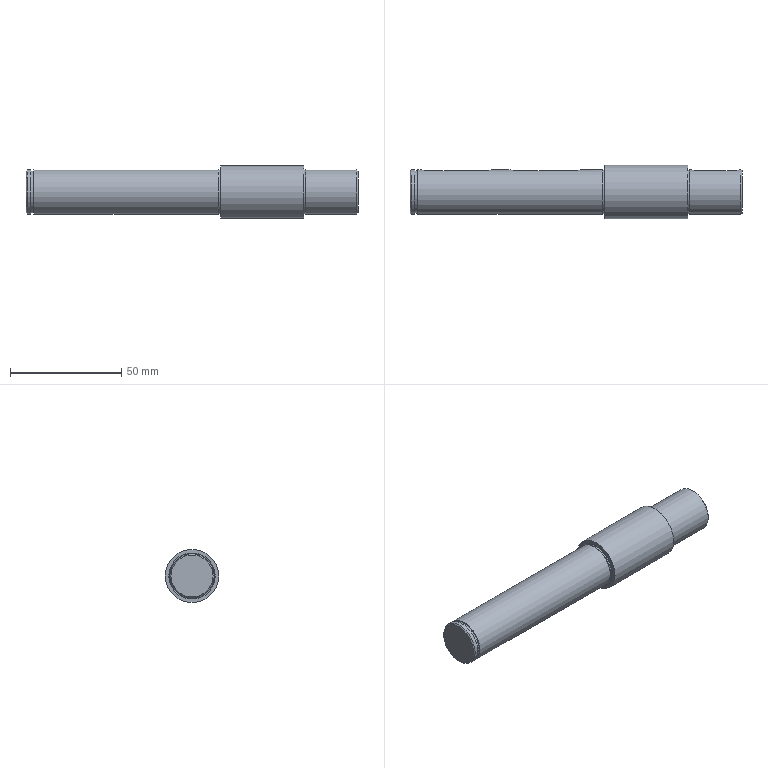Part | STEP file | Shaft1 | 1 solid | 41 faces | box 149.35 x 24 x 24 mm | volume 50304 mm3 | plane 16 | cylinder 14 | cone 7 | torus 4 | commonest cylinder face diameters 6 x6 20 x3 19.8 x2 6.8 x1 19 x1 24 x1